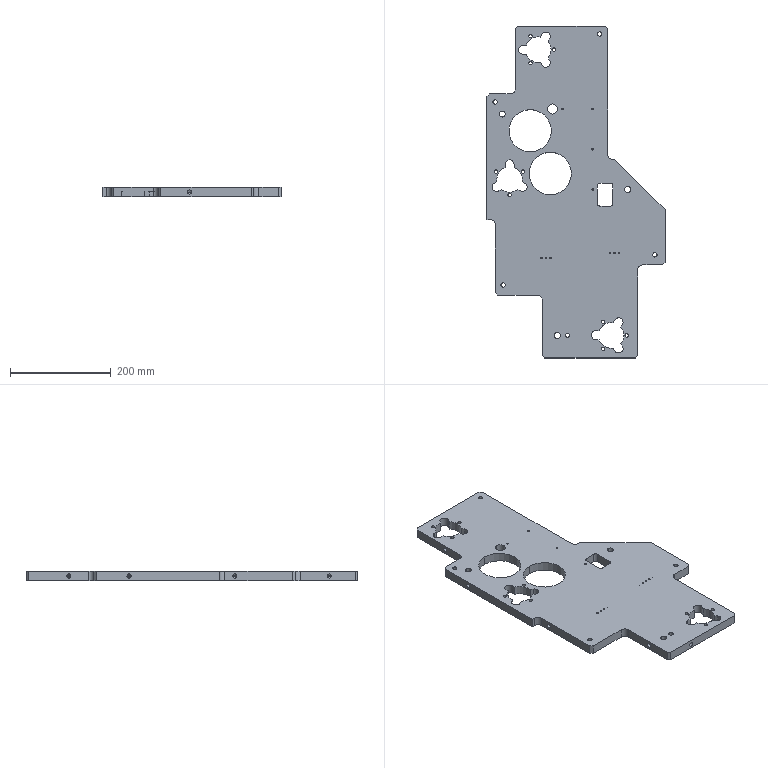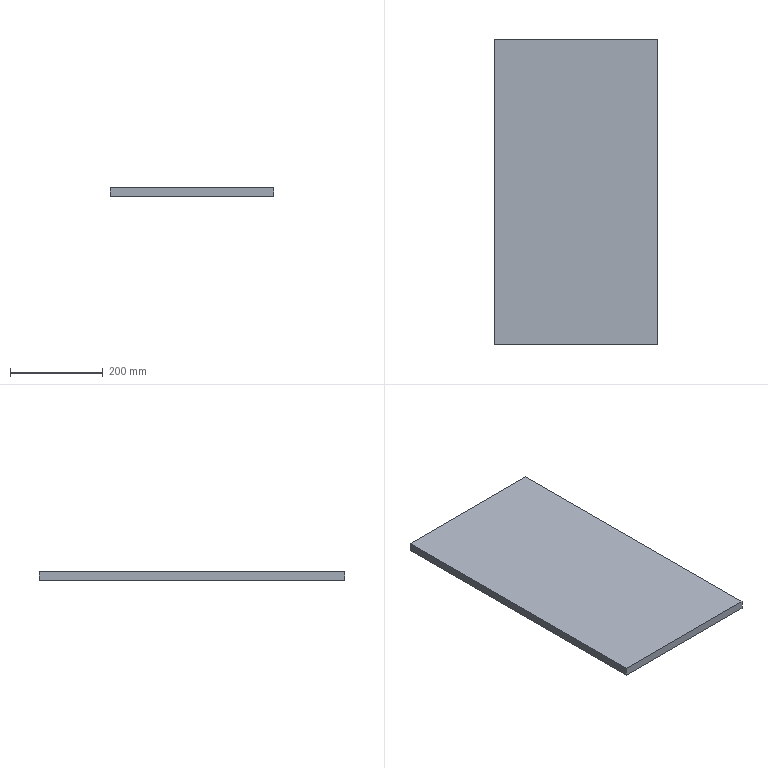CAM job | NX | 3-axis milling, drilling | part box 354 x 660 x 18 mm | stock box 354 x 660 x 18 mm
Tools:
number,name,description,diameter,corner_radius,flute_length,length,flutes
1,ZXZ,Milling Tool-5 Parameters,6.0,0.0,50.0,75.0,2
6,6.8ZT,Drilling Tool,6.8,0.0,35.0,50.0,2
8,D8C,Milling Tool-5 Parameters,8.0,0.0,50.0,75.0,2
9,D8JING,Milling Tool-5 Parameters,8.0,0.0,50.0,75.0,2
7,D6A45,Milling Tool-5 Parameters,6.0,0.0,50.0,75.0,2
13,3.3ZT,Drilling Tool,3.3,0.0,35.0,50.0,2
12,3.8ZT,Drilling Tool,3.8,0.0,35.0,50.0,2
14,4.2ZT,Drilling Tool,4.2,0.0,35.0,50.0,2
2,4.8ZT,Drilling Tool,4.8,0.0,35.0,50.0,2
3,D3,Milling Tool-5 Parameters,3.0,0.0,50.0,75.0,2
11,8.5ZT,Drilling Tool,8.5,0.0,35.0,50.0,2
10,12.0ZT,Drilling Tool,12.0,0.0,35.0,50.0,2
4,D4,Milling Tool-5 Parameters,4.0,0.0,50.0,75.0,2
Operations:
program,operation,operation_type,tool,method,geometry_group,spindle_rpm,surface_speed,feed_per_tooth,feed_cut,feed_plunge,cut_length_mm,path_length_mm,cut_time_min,machine_time_min
1,DRILLING,Operation,ZXZ,METHOD,A,3000.0,56.0,0.0417,250.0,0.0,36.0,1008.247,0.144,0.2412
1,DRILLING_COPY,Operation,6.8ZT,METHOD,A,2000.0,42.0,0.0375,150.0,0.0,220.886,1378.02,1.473,1.588
1,ZLEVEL_PROFILE,ZLevelMilling,D8C,METHOD,A,4000.0,100.0,0.3125,2500.0,1000.0,196874.627,198304.557,78.842,78.985
1,ZLEVEL_PROFILE_COPY,ZLevelMilling,D8C,METHOD,A,4000.0,100.0,0.3125,2500.0,1000.0,390620.99,390697.69,156.268,156.276
1,ZLEVEL_PROFILE_COPY_1,ZLevelMilling,D8JING,METHOD,A,6000.0,150.0,0.0833,1000.0,1000.0,1105.48,2342.409,1.105,1.229
1,ZLEVEL_PROFILE_COPY_COPY,ZLevelMilling,D8JING,METHOD,A,6000.0,150.0,0.0833,1000.0,1000.0,1957.097,2054.897,1.957,1.967
1,PLANAR_MILL,PlanarMilling,D6A45,METHOD,A,7500.0,141.0,0.0833,1250.0,100.0,1416.008,3169.727,1.133,1.308
1,FACE_MILLING,FaceMilling,D8JING,METHOD,A,6500.0,163.0,0.0962,1250.0,100.0,43794.285,43848.285,35.035,35.041
2,FACE_MILLING_COPY,FaceMilling,D8JING,METHOD,B,6500.0,163.0,0.0962,1250.0,100.0,43794.285,43848.285,35.035,35.041
2,PLANAR_MILL_COPY,PlanarMilling,D6A45,METHOD,B,7500.0,141.0,0.0833,1250.0,100.0,1416.008,3162.964,1.133,1.308
11铣右边,DRILLING_COPY_1,Operation,ZXZ,METHOD,AA,3000.0,56.0,0.0417,250.0,0.0,24.0,634.281,0.096,0.157
11铣右边,DRILLING_COPY_COPY,Operation,6.8ZT,METHOD,AA,2000.0,42.0,0.0375,150.0,0.0,147.258,880.796,0.9817,1.055
11铣右边,ZLEVEL_PROFILE_COPY_2,ZLevelMilling,D8C,METHOD,AA,4000.0,100.0,0.3125,2500.0,1000.0,160206.202,161257.872,64.156,64.261
11铣右边,ZLEVEL_PROFILE_COPY_COPY_1,ZLevelMilling,D8C,METHOD,AA,4000.0,100.0,0.3125,2500.0,1000.0,226482.457,226656.257,91.552,91.57
11铣右边,ZLEVEL_PROFILE_COPY_1_COPY,ZLevelMilling,D8JING,METHOD,AA,6000.0,150.0,0.0833,1000.0,1000.0,899.171,1975.188,0.8992,1.007
11铣右边,ZLEVEL_PROFILE_COPY_COPY_COPY,ZLevelMilling,D8JING,METHOD,AA,6000.0,150.0,0.0833,1000.0,1000.0,1120.865,1298.665,1.121,1.139
11铣右边,PLANAR_MILL_COPY_1,PlanarMilling,D6A45,METHOD,AA,7500.0,141.0,0.0833,1250.0,100.0,1120.671,3022.945,0.8965,1.087
11铣右边,FACE_MILLING_COPY_1,FaceMilling,D8JING,METHOD,AA,6500.0,163.0,0.0962,1250.0,100.0,26600.898,26734.898,21.281,21.294
铣右边,DRILLING_COPY_1_COPY,Operation,ZXZ,METHOD,AA,3000.0,56.0,0.0417,250.0,0.0,292.0,2859.085,1.168,1.425
铣右边,DRILLING_COPY_COPY_COPY_2_COPY,Operation,3.3ZT,METHOD,AA,2000.0,20.0,0.03,120.0,0.0,478.908,2331.865,3.991,4.176
铣右边,DRILLING_COPY_COPY_COPY_2,Operation,4.2ZT,METHOD,AA,2000.0,42.0,0.0375,150.0,0.0,233.265,1211,1.555,1.653
铣右边,DRILLING_COPY_COPY_COPY_2_COPY_COPY,Operation,3.8ZT,METHOD,AA,2000.0,20.0,0.03,120.0,0.0,162.266,1104.764,1.352,1.446
铣右边,DRILLING_COPY_COPY_COPY_COPY,Operation,4.8ZT,METHOD,AA,2000.0,42.0,0.0375,150.0,0.0,49.768,444.425,0.3318,0.3713
铣右边,DRILLING_COPY_COPY_COPY_1_COPY,Operation,8.5ZT,METHOD,AA,1573.0,42.0,0.0477,150.0,0.0,50.107,491.202,0.334,0.3782
铣右边,DRILLING_COPY_COPY_COPY_1_COPY_COPY,Operation,12.0ZT,METHOD,AA,1200.0,45.0,0.0625,150.0,0.0,78.316,622.512,0.5221,0.5765
铣右边,HOLE_MILLING,CylinderMilling,D8C,METHOD,AA,4000.0,100.0,0.1875,1500.0,100.0,14005.232,14162.732,9.337,9.353
铣右边,ZLEVEL_PROFILE_COPY_2_COPY,ZLevelMilling,D8C,METHOD,AA,4000.0,100.0,0.3125,2500.0,1000.0,21272.382,21427.382,8.527,8.543
铣右边,ZLEVEL_PROFILE_COPY_1_COPY_COPY_1,ZLevelMilling,D8JING,METHOD,AA,6000.0,150.0,0.0833,1000.0,1000.0,165.649,708.466,0.1656,0.2199
铣右边,PLANAR_MILL_COPY_1_COPY_1,PlanarMilling,D6A45,METHOD,AA,7500.0,141.0,0.0833,1250.0,100.0,2422.646,16467.55,1.938,3.343
铣右边,刀补4,CylinderMilling,D4,METHOD,AA,5000.0,47.0,0.085,850.0,100.0,148.863,924.541,0.1751,0.2527
铣右边,刀补4_COPY,CylinderMilling,D3,METHOD,AA,5000.0,47.0,0.085,850.0,100.0,499.483,3381.106,0.5876,0.8758
11接左边,DRILLING_COPY_2,Operation,ZXZ,METHOD,BB,3000.0,56.0,0.0417,250.0,0.0,12.0,277.555,0.048,0.0746
11接左边,DRILLING_COPY_COPY_1,Operation,6.8ZT,METHOD,BB,2000.0,42.0,0.0375,150.0,0.0,73.629,400.812,0.4909,0.5236
11接左边,ZLEVEL_PROFILE_COPY_3,ZLevelMilling,D8C,METHOD,BB,4000.0,100.0,0.3125,2500.0,1000.0,36667.189,36821.989,14.685,14.701
11接左边,ZLEVEL_PROFILE_COPY_COPY_1_COPY,ZLevelMilling,D8C,METHOD,BB,4000.0,100.0,0.3125,2500.0,1000.0,186115.127,186288.927,75.377,75.394
11接左边,ZLEVEL_PROFILE_COPY_1_COPY_COPY,ZLevelMilling,D8JING,METHOD,BB,6000.0,150.0,0.0833,1000.0,1000.0,206.31,380.31,0.2063,0.2237
11接左边,ZLEVEL_PROFILE_COPY_COPY_COPY_COPY,ZLevelMilling,D8JING,METHOD,BB,6000.0,150.0,0.0833,1000.0,1000.0,919.317,1097.117,0.9193,0.9371
11接左边,PLANAR_MILL_COPY_1_COPY,PlanarMilling,D6A45,METHOD,BB,7500.0,141.0,0.0833,1250.0,100.0,295.338,962.949,0.2363,0.303
11接左边,FACE_MILLING_COPY_1_COPY,FaceMilling,D8JING,METHOD,BB,6500.0,163.0,0.0962,1250.0,100.0,18689.979,18823.979,14.952,14.965
铣左边,DRILLING_COPY_2_COPY,Operation,ZXZ,METHOD,BB,3000.0,56.0,0.0417,250.0,0.0,264.0,2406.022,1.056,1.27
铣左边,DRILLING_COPY_COPY_COPY_2_COPY_COPY_1,Operation,3.3ZT,METHOD,BB,2000.0,20.0,0.03,120.0,0.0,704.605,3069.205,5.872,6.108
铣左边,DRILLING_COPY_COPY_COPY_2_COPY_1,Operation,4.2ZT,METHOD,BB,2000.0,42.0,0.0375,150.0,0.0,49.985,302.291,0.3332,0.3585
铣左边,DRILLING_COPY_COPY_COPY_2_COPY_COPY_COPY,Operation,3.8ZT,METHOD,BB,2000.0,20.0,0.03,120.0,0.0,169.841,1059.094,1.415,1.504
铣左边,DRILLING_COPY_COPY_COPY_1_COPY_COPY_1,Operation,8.5ZT,METHOD,BB,1573.0,42.0,0.0477,150.0,0.0,75.161,695.181,0.5011,0.5631
铣左边,DRILLING_COPY_COPY_COPY_1_COPY_COPY_COPY,Operation,12.0ZT,METHOD,BB,1200.0,45.0,0.0625,150.0,0.0,26.105,192.21,0.174,0.1906
铣左边,FLOOR_WALL,VolumeBased25DMillingOperation,D8C,METHOD,BB,4000.0,100.0,0.25,2000.0,1000.0,175014.198,181409.536,90.381,91.02
铣左边,FLOOR_WALL_COPY,VolumeBased25DMillingOperation,D8JING,METHOD,BB,5000.0,125.0,0.1,1000.0,1000.0,2888.43,3287.566,2.888,2.928
铣左边,PLANAR_MILL_COPY_1_COPY_1_COPY,PlanarMilling,D6A45,METHOD,BB,7500.0,141.0,0.0833,1250.0,100.0,1684.737,11877.012,1.348,2.367
铣左边,刀补3_COPY_COPY,CylinderMilling,D3,METHOD,BB,5000.0,47.0,0.085,850.0,100.0,405.83,2873.773,0.4774,0.7242
22铣左边,FACE_MILLING_COPY_COPY,FaceMilling,D8JING,METHOD,CC,6500.0,163.0,0.0962,1250.0,100.0,26601.562,26735.562,21.281,21.295
22铣左边,PLANAR_MILL_COPY_COPY,PlanarMilling,D6A45,METHOD,CC,7500.0,141.0,0.0833,1250.0,100.0,1120.671,3013.185,0.8965,1.086
22接右边,FACE_MILLING_COPY_COPY_COPY,FaceMilling,D8JING,METHOD,DD,6500.0,163.0,0.0962,1250.0,100.0,18816.21,18950.21,15.053,15.066
22接右边,PLANAR_MILL_COPY_COPY_COPY,PlanarMilling,D6A45,METHOD,DD,7500.0,141.0,0.0833,1250.0,100.0,295.338,966.163,0.2363,0.3034
背面,DRILLING_COPY_2_COPY_COPY,Operation,ZXZ,METHOD,EE,3000.0,56.0,0.0417,250.0,0.0,16.0,321.187,0.064,0.0945
背面,DRILLING_COPY_COPY_COPY_2_COPY_COPY_1_COPY,Operation,3.3ZT,METHOD,EE,2000.0,20.0,0.03,120.0,0.0,56.366,401.919,0.4697,0.5043
第1铣,FACE_MILLING_COPY_COPY_COPY_1,FaceMilling,D8JING,METHOD,F,6500.0,163.0,0.0962,1250.0,100.0,56979.654,57033.654,45.584,45.589
第2铣,FACE_MILLING_COPY_COPY_COPY_1_COPY,FaceMilling,D8JING,METHOD,G,6500.0,163.0,0.0962,1250.0,100.0,15595.117,15649.117,12.476,12.482